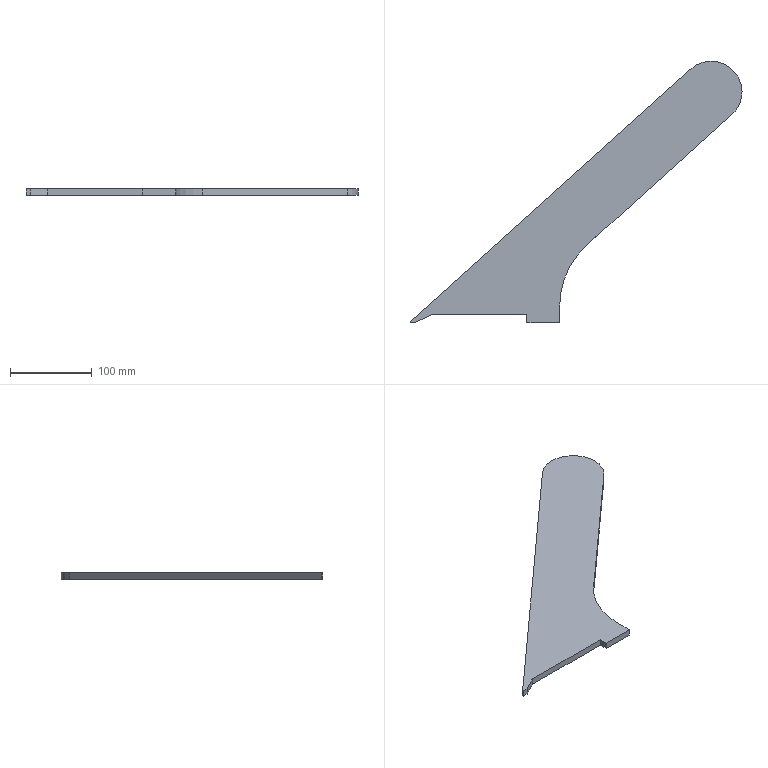Part | SolidWorks | features FlatPattern 1, SMBaseFlange 1, SheetMetal 1 | 1 solid | 14 faces | box 405.176 x 319.37 x 8 mm | volume 281277 mm3 | plane 11 | cylinder 3 | commonest cylinder face diameters 75 x2 200 x1
STEP:
#1=CARTESIAN_POINT('',(430.152,288.015,-8.));
#2=VERTEX_POINT('',#1);
#3=CARTESIAN_POINT('',(442.571,315.893,-8.));
#4=VERTEX_POINT('',#3);
#5=CARTESIAN_POINT('',(405.071,315.893,-8.));
#6=DIRECTION('',(0.,0.,1.));
#7=DIRECTION('',(1.,0.,0.));
#8=AXIS2_PLACEMENT_3D('',#5,#6,#7);
#9=CIRCLE('',#8,37.5);
#10=EDGE_CURVE('',#2,#4,#9,.T.);
#11=ORIENTED_EDGE('',*,*,#10,.T.);
#12=CARTESIAN_POINT('',(442.571,315.893,0.));
#13=VERTEX_POINT('',#12);
#14=CARTESIAN_POINT('',(442.571,315.893,-8.));
#15=DIRECTION('',(0.,0.,1.));
#16=VECTOR('',#15,1000.);
#17=LINE('',#14,#16);
#18=EDGE_CURVE('',#4,#13,#17,.T.);
#19=ORIENTED_EDGE('',*,*,#18,.T.);
#20=CARTESIAN_POINT('',(430.152,288.015,0.));
#21=VERTEX_POINT('',#20);
#22=CARTESIAN_POINT('',(405.071,315.893,0.));
#23=DIRECTION('',(0.,0.,1.));
#24=DIRECTION('',(1.,0.,0.));
#25=AXIS2_PLACEMENT_3D('',#22,#23,#24);
#26=CIRCLE('',#25,37.5);
#27=EDGE_CURVE('',#21,#13,#26,.T.);
#28=ORIENTED_EDGE('',*,*,#27,.F.);
#29=CARTESIAN_POINT('',(430.152,288.015,-8.));
#30=DIRECTION('',(0.,0.,1.));
#31=VECTOR('',#30,1000.);
#32=LINE('',#29,#31);
#33=EDGE_CURVE('',#2,#21,#32,.T.);
#34=ORIENTED_EDGE('',*,*,#33,.F.);
#35=EDGE_LOOP('',(#11,#19,#28,#34));
#36=FACE_OUTER_BOUND('',#35,.T.);
#37=CARTESIAN_POINT('',(405.071,315.893,-8.));
#38=DIRECTION('',(0.,0.,1.));
#39=DIRECTION('',(1.,0.,0.));
#40=AXIS2_PLACEMENT_3D('',#37,#38,#39);
#41=CYLINDRICAL_SURFACE('',#40,37.5);
#42=ADVANCED_FACE('',(#36),#41,.T.);
#43=CARTESIAN_POINT('',(220.081,54.476,0.));
#44=VERTEX_POINT('',#43);
#45=CARTESIAN_POINT('',(253.198,128.818,0.));
#46=VERTEX_POINT('',#45);
#47=CARTESIAN_POINT('',(320.081,54.476,0.));
#48=DIRECTION('',(0.,0.,-1.));
#49=DIRECTION('',(1.,0.,0.));
#50=AXIS2_PLACEMENT_3D('',#47,#48,#49);
#51=CIRCLE('',#50,100.);
#52=EDGE_CURVE('',#44,#46,#51,.T.);
#53=ORIENTED_EDGE('',*,*,#52,.F.);
#54=CARTESIAN_POINT('',(220.081,54.476,-8.));
#55=VERTEX_POINT('',#54);
#56=CARTESIAN_POINT('',(220.081,54.476,-8.));
#57=DIRECTION('',(0.,0.,1.));
#58=VECTOR('',#57,1000.);
#59=LINE('',#56,#58);
#60=EDGE_CURVE('',#55,#44,#59,.T.);
#61=ORIENTED_EDGE('',*,*,#60,.F.);
#62=CARTESIAN_POINT('',(253.198,128.818,-8.));
#63=VERTEX_POINT('',#62);
#64=CARTESIAN_POINT('',(320.081,54.476,-8.));
#65=DIRECTION('',(0.,0.,-1.));
#66=DIRECTION('',(1.,0.,0.));
#67=AXIS2_PLACEMENT_3D('',#64,#65,#66);
#68=CIRCLE('',#67,100.);
#69=EDGE_CURVE('',#55,#63,#68,.T.);
#70=ORIENTED_EDGE('',*,*,#69,.T.);
#71=CARTESIAN_POINT('',(253.198,128.818,-8.));
#72=DIRECTION('',(0.,0.,1.));
#73=VECTOR('',#72,1000.);
#74=LINE('',#71,#73);
#75=EDGE_CURVE('',#63,#46,#74,.T.);
#76=ORIENTED_EDGE('',*,*,#75,.T.);
#77=EDGE_LOOP('',(#53,#61,#70,#76));
#78=FACE_OUTER_BOUND('',#77,.T.);
#79=CARTESIAN_POINT('',(320.081,54.476,-8.));
#80=DIRECTION('',(0.,0.,1.));
#81=DIRECTION('',(1.,0.,0.));
#82=AXIS2_PLACEMENT_3D('',#79,#80,#81);
#83=CYLINDRICAL_SURFACE('',#82,100.);
#84=ADVANCED_FACE('',(#78),#83,.F.);
#85=CARTESIAN_POINT('',(220.081,34.023,0.));
#86=VERTEX_POINT('',#85);
#87=CARTESIAN_POINT('',(220.081,34.023,0.));
#88=DIRECTION('',(0.,1.,0.));
#89=VECTOR('',#88,1000.);
#90=LINE('',#87,#89);
#91=EDGE_CURVE('',#86,#44,#90,.T.);
#92=ORIENTED_EDGE('',*,*,#91,.F.);
#93=CARTESIAN_POINT('',(220.081,34.023,-8.));
#94=VERTEX_POINT('',#93);
#95=CARTESIAN_POINT('',(220.081,34.023,-8.));
#96=DIRECTION('',(0.,0.,1.));
#97=VECTOR('',#96,1000.);
#98=LINE('',#95,#97);
#99=EDGE_CURVE('',#94,#86,#98,.T.);
#100=ORIENTED_EDGE('',*,*,#99,.F.);
#101=CARTESIAN_POINT('',(220.081,34.023,-8.));
#102=DIRECTION('',(0.,1.,0.));
#103=VECTOR('',#102,1000.);
#104=LINE('',#101,#103);
#105=EDGE_CURVE('',#94,#55,#104,.T.);
#106=ORIENTED_EDGE('',*,*,#105,.T.);
#107=ORIENTED_EDGE('',*,*,#60,.T.);
#108=EDGE_LOOP('',(#92,#100,#106,#107));
#109=FACE_OUTER_BOUND('',#108,.T.);
#110=CARTESIAN_POINT('',(220.081,34.023,-8.));
#111=DIRECTION('',(1.,0.,0.));
#112=DIRECTION('',(0.,0.,-1.));
#113=AXIS2_PLACEMENT_3D('',#110,#111,#112);
#114=PLANE('',#113);
#115=ADVANCED_FACE('',(#109),#114,.T.);
#116=CARTESIAN_POINT('',(180.081,34.023,0.));
#117=VERTEX_POINT('',#116);
#118=CARTESIAN_POINT('',(180.081,34.023,0.));
#119=DIRECTION('',(1.,0.,0.));
#120=VECTOR('',#119,1000.);
#121=LINE('',#118,#120);
#122=EDGE_CURVE('',#117,#86,#121,.T.);
#123=ORIENTED_EDGE('',*,*,#122,.F.);
#124=CARTESIAN_POINT('',(180.081,34.023,-8.));
#125=VERTEX_POINT('',#124);
#126=CARTESIAN_POINT('',(180.081,34.023,-8.));
#127=DIRECTION('',(0.,0.,1.));
#128=VECTOR('',#127,1000.);
#129=LINE('',#126,#128);
#130=EDGE_CURVE('',#125,#117,#129,.T.);
#131=ORIENTED_EDGE('',*,*,#130,.F.);
#132=CARTESIAN_POINT('',(180.081,34.023,-8.));
#133=DIRECTION('',(1.,0.,0.));
#134=VECTOR('',#133,1000.);
#135=LINE('',#132,#134);
#136=EDGE_CURVE('',#125,#94,#135,.T.);
#137=ORIENTED_EDGE('',*,*,#136,.T.);
#138=ORIENTED_EDGE('',*,*,#99,.T.);
#139=EDGE_LOOP('',(#123,#131,#137,#138));
#140=FACE_OUTER_BOUND('',#139,.T.);
#141=CARTESIAN_POINT('',(180.081,34.023,-8.));
#142=DIRECTION('',(0.,-1.,0.));
#143=DIRECTION('',(1.,0.,0.));
#144=AXIS2_PLACEMENT_3D('',#141,#142,#143);
#145=PLANE('',#144);
#146=ADVANCED_FACE('',(#140),#145,.T.);
#147=CARTESIAN_POINT('',(180.081,44.023,0.));
#148=VERTEX_POINT('',#147);
#149=CARTESIAN_POINT('',(180.081,44.023,0.));
#150=DIRECTION('',(0.,-1.,0.));
#151=VECTOR('',#150,1000.);
#152=LINE('',#149,#151);
#153=EDGE_CURVE('',#148,#117,#152,.T.);
#154=ORIENTED_EDGE('',*,*,#153,.F.);
#155=CARTESIAN_POINT('',(180.081,44.023,-8.));
#156=VERTEX_POINT('',#155);
#157=CARTESIAN_POINT('',(180.081,44.023,-8.));
#158=DIRECTION('',(0.,0.,1.));
#159=VECTOR('',#158,1000.);
#160=LINE('',#157,#159);
#161=EDGE_CURVE('',#156,#148,#160,.T.);
#162=ORIENTED_EDGE('',*,*,#161,.F.);
#163=CARTESIAN_POINT('',(180.081,44.023,-8.));
#164=DIRECTION('',(0.,-1.,0.));
#165=VECTOR('',#164,1000.);
#166=LINE('',#163,#165);
#167=EDGE_CURVE('',#156,#125,#166,.T.);
#168=ORIENTED_EDGE('',*,*,#167,.T.);
#169=ORIENTED_EDGE('',*,*,#130,.T.);
#170=EDGE_LOOP('',(#154,#162,#168,#169));
#171=FACE_OUTER_BOUND('',#170,.T.);
#172=CARTESIAN_POINT('',(180.081,44.023,-8.));
#173=DIRECTION('',(-1.,0.,0.));
#174=DIRECTION('',(0.,0.,1.));
#175=AXIS2_PLACEMENT_3D('',#172,#173,#174);
#176=PLANE('',#175);
#177=ADVANCED_FACE('',(#171),#176,.T.);
#178=CARTESIAN_POINT('',(63.081,44.023,0.));
#179=VERTEX_POINT('',#178);
#180=CARTESIAN_POINT('',(63.081,44.023,0.));
#181=DIRECTION('',(1.,0.,0.));
#182=VECTOR('',#181,1000.);
#183=LINE('',#180,#182);
#184=EDGE_CURVE('',#179,#148,#183,.T.);
#185=ORIENTED_EDGE('',*,*,#184,.F.);
#186=CARTESIAN_POINT('',(63.081,44.023,-8.));
#187=VERTEX_POINT('',#186);
#188=CARTESIAN_POINT('',(63.081,44.023,-8.));
#189=DIRECTION('',(0.,0.,1.));
#190=VECTOR('',#189,1000.);
#191=LINE('',#188,#190);
#192=EDGE_CURVE('',#187,#179,#191,.T.);
#193=ORIENTED_EDGE('',*,*,#192,.F.);
#194=CARTESIAN_POINT('',(63.081,44.023,-8.));
#195=DIRECTION('',(1.,0.,0.));
#196=VECTOR('',#195,1000.);
#197=LINE('',#194,#196);
#198=EDGE_CURVE('',#187,#156,#197,.T.);
#199=ORIENTED_EDGE('',*,*,#198,.T.);
#200=ORIENTED_EDGE('',*,*,#161,.T.);
#201=EDGE_LOOP('',(#185,#193,#199,#200));
#202=FACE_OUTER_BOUND('',#201,.T.);
#203=CARTESIAN_POINT('',(63.081,44.023,-8.));
#204=DIRECTION('',(0.,-1.,0.));
#205=DIRECTION('',(0.,0.,-1.));
#206=AXIS2_PLACEMENT_3D('',#203,#204,#205);
#207=PLANE('',#206);
#208=ADVANCED_FACE('',(#202),#207,.T.);
#209=CARTESIAN_POINT('',(43.455,34.023,0.));
#210=VERTEX_POINT('',#209);
#211=CARTESIAN_POINT('',(43.455,34.023,0.));
#212=DIRECTION('',(0.891,0.454,0.));
#213=VECTOR('',#212,1000.);
#214=LINE('',#211,#213);
#215=EDGE_CURVE('',#210,#179,#214,.T.);
#216=ORIENTED_EDGE('',*,*,#215,.F.);
#217=CARTESIAN_POINT('',(43.455,34.023,-8.));
#218=VERTEX_POINT('',#217);
#219=CARTESIAN_POINT('',(43.455,34.023,-8.));
#220=DIRECTION('',(0.,0.,1.));
#221=VECTOR('',#220,1000.);
#222=LINE('',#219,#221);
#223=EDGE_CURVE('',#218,#210,#222,.T.);
#224=ORIENTED_EDGE('',*,*,#223,.F.);
#225=CARTESIAN_POINT('',(43.455,34.023,-8.));
#226=DIRECTION('',(0.891,0.454,0.));
#227=VECTOR('',#226,1000.);
#228=LINE('',#225,#227);
#229=EDGE_CURVE('',#218,#187,#228,.T.);
#230=ORIENTED_EDGE('',*,*,#229,.T.);
#231=ORIENTED_EDGE('',*,*,#192,.T.);
#232=EDGE_LOOP('',(#216,#224,#230,#231));
#233=FACE_OUTER_BOUND('',#232,.T.);
#234=CARTESIAN_POINT('',(43.455,34.023,-8.));
#235=DIRECTION('',(0.454,-0.891,0.));
#236=DIRECTION('',(0.891,0.454,0.));
#237=AXIS2_PLACEMENT_3D('',#234,#235,#236);
#238=PLANE('',#237);
#239=ADVANCED_FACE('',(#233),#238,.T.);
#240=CARTESIAN_POINT('',(37.395,34.023,0.));
#241=VERTEX_POINT('',#240);
#242=CARTESIAN_POINT('',(37.395,34.023,0.));
#243=DIRECTION('',(1.,0.,0.));
#244=VECTOR('',#243,1000.);
#245=LINE('',#242,#244);
#246=EDGE_CURVE('',#241,#210,#245,.T.);
#247=ORIENTED_EDGE('',*,*,#246,.F.);
#248=CARTESIAN_POINT('',(37.395,34.023,-8.));
#249=VERTEX_POINT('',#248);
#250=CARTESIAN_POINT('',(37.395,34.023,-8.));
#251=DIRECTION('',(0.,0.,1.));
#252=VECTOR('',#251,1000.);
#253=LINE('',#250,#252);
#254=EDGE_CURVE('',#249,#241,#253,.T.);
#255=ORIENTED_EDGE('',*,*,#254,.F.);
#256=CARTESIAN_POINT('',(37.395,34.023,-8.));
#257=DIRECTION('',(1.,0.,0.));
#258=VECTOR('',#257,1000.);
#259=LINE('',#256,#258);
#260=EDGE_CURVE('',#249,#218,#259,.T.);
#261=ORIENTED_EDGE('',*,*,#260,.T.);
#262=ORIENTED_EDGE('',*,*,#223,.T.);
#263=EDGE_LOOP('',(#247,#255,#261,#262));
#264=FACE_OUTER_BOUND('',#263,.T.);
#265=CARTESIAN_POINT('',(37.395,34.023,-8.));
#266=DIRECTION('',(0.,-1.,0.));
#267=DIRECTION('',(0.,0.,-1.));
#268=AXIS2_PLACEMENT_3D('',#265,#266,#267);
#269=PLANE('',#268);
#270=ADVANCED_FACE('',(#264),#269,.T.);
#271=CARTESIAN_POINT('',(37.395,35.553,0.));
#272=VERTEX_POINT('',#271);
#273=CARTESIAN_POINT('',(37.395,35.553,0.));
#274=DIRECTION('',(0.,-1.,0.));
#275=VECTOR('',#274,1000.);
#276=LINE('',#273,#275);
#277=EDGE_CURVE('',#272,#241,#276,.T.);
#278=ORIENTED_EDGE('',*,*,#277,.F.);
#279=CARTESIAN_POINT('',(37.395,35.553,-8.));
#280=VERTEX_POINT('',#279);
#281=CARTESIAN_POINT('',(37.395,35.553,-8.));
#282=DIRECTION('',(0.,0.,1.));
#283=VECTOR('',#282,1000.);
#284=LINE('',#281,#283);
#285=EDGE_CURVE('',#280,#272,#284,.T.);
#286=ORIENTED_EDGE('',*,*,#285,.F.);
#287=CARTESIAN_POINT('',(37.395,35.553,-8.));
#288=DIRECTION('',(0.,-1.,0.));
#289=VECTOR('',#288,1000.);
#290=LINE('',#287,#289);
#291=EDGE_CURVE('',#280,#249,#290,.T.);
#292=ORIENTED_EDGE('',*,*,#291,.T.);
#293=ORIENTED_EDGE('',*,*,#254,.T.);
#294=EDGE_LOOP('',(#278,#286,#292,#293));
#295=FACE_OUTER_BOUND('',#294,.T.);
#296=CARTESIAN_POINT('',(37.395,35.553,-8.));
#297=DIRECTION('',(-1.,0.,0.));
#298=DIRECTION('',(0.,0.,1.));
#299=AXIS2_PLACEMENT_3D('',#296,#297,#298);
#300=PLANE('',#299);
#301=ADVANCED_FACE('',(#295),#300,.T.);
#302=CARTESIAN_POINT('',(379.99,343.772,0.));
#303=VERTEX_POINT('',#302);
#304=CARTESIAN_POINT('',(379.99,343.772,0.));
#305=DIRECTION('',(-0.7434,-0.6688,0.));
#306=VECTOR('',#305,1000.);
#307=LINE('',#304,#306);
#308=EDGE_CURVE('',#303,#272,#307,.T.);
#309=ORIENTED_EDGE('',*,*,#308,.F.);
#310=CARTESIAN_POINT('',(379.99,343.772,-8.));
#311=VERTEX_POINT('',#310);
#312=CARTESIAN_POINT('',(379.99,343.772,-8.));
#313=DIRECTION('',(0.,0.,1.));
#314=VECTOR('',#313,1000.);
#315=LINE('',#312,#314);
#316=EDGE_CURVE('',#311,#303,#315,.T.);
#317=ORIENTED_EDGE('',*,*,#316,.F.);
#318=CARTESIAN_POINT('',(379.99,343.772,-8.));
#319=DIRECTION('',(-0.7434,-0.6688,0.));
#320=VECTOR('',#319,1000.);
#321=LINE('',#318,#320);
#322=EDGE_CURVE('',#311,#280,#321,.T.);
#323=ORIENTED_EDGE('',*,*,#322,.T.);
#324=ORIENTED_EDGE('',*,*,#285,.T.);
#325=EDGE_LOOP('',(#309,#317,#323,#324));
#326=FACE_OUTER_BOUND('',#325,.T.);
#327=CARTESIAN_POINT('',(379.99,343.772,-8.));
#328=DIRECTION('',(-0.6688,0.7434,0.));
#329=DIRECTION('',(-0.7434,-0.6688,0.));
#330=AXIS2_PLACEMENT_3D('',#327,#328,#329);
#331=PLANE('',#330);
#332=ADVANCED_FACE('',(#326),#331,.T.);
#333=ORIENTED_EDGE('',*,*,#18,.F.);
#334=CARTESIAN_POINT('',(405.071,315.893,-8.));
#335=DIRECTION('',(0.,0.,1.));
#336=DIRECTION('',(1.,0.,0.));
#337=AXIS2_PLACEMENT_3D('',#334,#335,#336);
#338=CIRCLE('',#337,37.5);
#339=EDGE_CURVE('',#4,#311,#338,.T.);
#340=ORIENTED_EDGE('',*,*,#339,.T.);
#341=ORIENTED_EDGE('',*,*,#316,.T.);
#342=CARTESIAN_POINT('',(405.071,315.893,0.));
#343=DIRECTION('',(0.,0.,1.));
#344=DIRECTION('',(1.,0.,0.));
#345=AXIS2_PLACEMENT_3D('',#342,#343,#344);
#346=CIRCLE('',#345,37.5);
#347=EDGE_CURVE('',#13,#303,#346,.T.);
#348=ORIENTED_EDGE('',*,*,#347,.F.);
#349=EDGE_LOOP('',(#333,#340,#341,#348));
#350=FACE_OUTER_BOUND('',#349,.T.);
#351=CARTESIAN_POINT('',(405.071,315.893,-8.));
#352=DIRECTION('',(0.,0.,1.));
#353=DIRECTION('',(1.,0.,0.));
#354=AXIS2_PLACEMENT_3D('',#351,#352,#353);
#355=CYLINDRICAL_SURFACE('',#354,37.5);
#356=ADVANCED_FACE('',(#350),#355,.T.);
#357=CARTESIAN_POINT('',(253.198,128.818,0.));
#358=DIRECTION('',(0.7434,0.6688,0.));
#359=VECTOR('',#358,1000.);
#360=LINE('',#357,#359);
#361=EDGE_CURVE('',#46,#21,#360,.T.);
#362=ORIENTED_EDGE('',*,*,#361,.F.);
#363=ORIENTED_EDGE('',*,*,#75,.F.);
#364=CARTESIAN_POINT('',(253.198,128.818,-8.));
#365=DIRECTION('',(0.7434,0.6688,0.));
#366=VECTOR('',#365,1000.);
#367=LINE('',#364,#366);
#368=EDGE_CURVE('',#63,#2,#367,.T.);
#369=ORIENTED_EDGE('',*,*,#368,.T.);
#370=ORIENTED_EDGE('',*,*,#33,.T.);
#371=EDGE_LOOP('',(#362,#363,#369,#370));
#372=FACE_OUTER_BOUND('',#371,.T.);
#373=CARTESIAN_POINT('',(253.198,128.818,-8.));
#374=DIRECTION('',(0.6688,-0.7434,0.));
#375=DIRECTION('',(0.7434,0.6688,0.));
#376=AXIS2_PLACEMENT_3D('',#373,#374,#375);
#377=PLANE('',#376);
#378=ADVANCED_FACE('',(#372),#377,.T.);
#379=ORIENTED_EDGE('',*,*,#69,.F.);
#380=ORIENTED_EDGE('',*,*,#105,.F.);
#381=ORIENTED_EDGE('',*,*,#136,.F.);
#382=ORIENTED_EDGE('',*,*,#167,.F.);
#383=ORIENTED_EDGE('',*,*,#198,.F.);
#384=ORIENTED_EDGE('',*,*,#229,.F.);
#385=ORIENTED_EDGE('',*,*,#260,.F.);
#386=ORIENTED_EDGE('',*,*,#291,.F.);
#387=ORIENTED_EDGE('',*,*,#322,.F.);
#388=ORIENTED_EDGE('',*,*,#339,.F.);
#389=ORIENTED_EDGE('',*,*,#10,.F.);
#390=ORIENTED_EDGE('',*,*,#368,.F.);
#391=EDGE_LOOP('',(#379,#380,#381,#382,#383,#384,#385,#386,#387,#388,#389,#390));
#392=FACE_OUTER_BOUND('',#391,.T.);
#393=CARTESIAN_POINT('',(320.081,54.476,-8.));
#394=DIRECTION('',(0.,0.,1.));
#395=DIRECTION('',(1.,0.,0.));
#396=AXIS2_PLACEMENT_3D('',#393,#394,#395);
#397=PLANE('',#396);
#398=ADVANCED_FACE('',(#392),#397,.F.);
#399=ORIENTED_EDGE('',*,*,#52,.T.);
#400=ORIENTED_EDGE('',*,*,#361,.T.);
#401=ORIENTED_EDGE('',*,*,#27,.T.);
#402=ORIENTED_EDGE('',*,*,#347,.T.);
#403=ORIENTED_EDGE('',*,*,#308,.T.);
#404=ORIENTED_EDGE('',*,*,#277,.T.);
#405=ORIENTED_EDGE('',*,*,#246,.T.);
#406=ORIENTED_EDGE('',*,*,#215,.T.);
#407=ORIENTED_EDGE('',*,*,#184,.T.);
#408=ORIENTED_EDGE('',*,*,#153,.T.);
#409=ORIENTED_EDGE('',*,*,#122,.T.);
#410=ORIENTED_EDGE('',*,*,#91,.T.);
#411=EDGE_LOOP('',(#399,#400,#401,#402,#403,#404,#405,#406,#407,#408,#409,#410));
#412=FACE_OUTER_BOUND('',#411,.T.);
#413=CARTESIAN_POINT('',(320.081,54.476,0.));
#414=DIRECTION('',(0.,0.,1.));
#415=DIRECTION('',(1.,0.,0.));
#416=AXIS2_PLACEMENT_3D('',#413,#414,#415);
#417=PLANE('',#416);
#418=ADVANCED_FACE('',(#412),#417,.T.);
#419=CLOSED_SHELL('',(#42,#84,#115,#146,#177,#208,#239,#270,#301,#332,#356,#378,#398,#418));
#420=MANIFOLD_SOLID_BREP('',#419);
#421=CARTESIAN_POINT('',(0.,0.,0.));
#422=DIRECTION('',(0.,0.,1.));
#423=DIRECTION('',(1.,0.,0.));
#424=AXIS2_PLACEMENT_3D('',#421,#422,#423);
#425=(LENGTH_UNIT()NAMED_UNIT(*)SI_UNIT(.MILLI.,.METRE.));
#426=UNCERTAINTY_MEASURE_WITH_UNIT(LENGTH_MEASURE(0.00001),#425,'','');
#427=(NAMED_UNIT(*)PLANE_ANGLE_UNIT()SI_UNIT($,.RADIAN.));
#428=(NAMED_UNIT(*)SI_UNIT($,.STERADIAN.)SOLID_ANGLE_UNIT());
#429=(GEOMETRIC_REPRESENTATION_CONTEXT(3)GLOBAL_UNCERTAINTY_ASSIGNED_CONTEXT((#426))GLOBAL_UNIT_ASSIGNED_CONTEXT((#425,#427,#428))REPRESENTATION_CONTEXT('',''));
#430=ADVANCED_BREP_SHAPE_REPRESENTATION('',(#420,#424),#429);